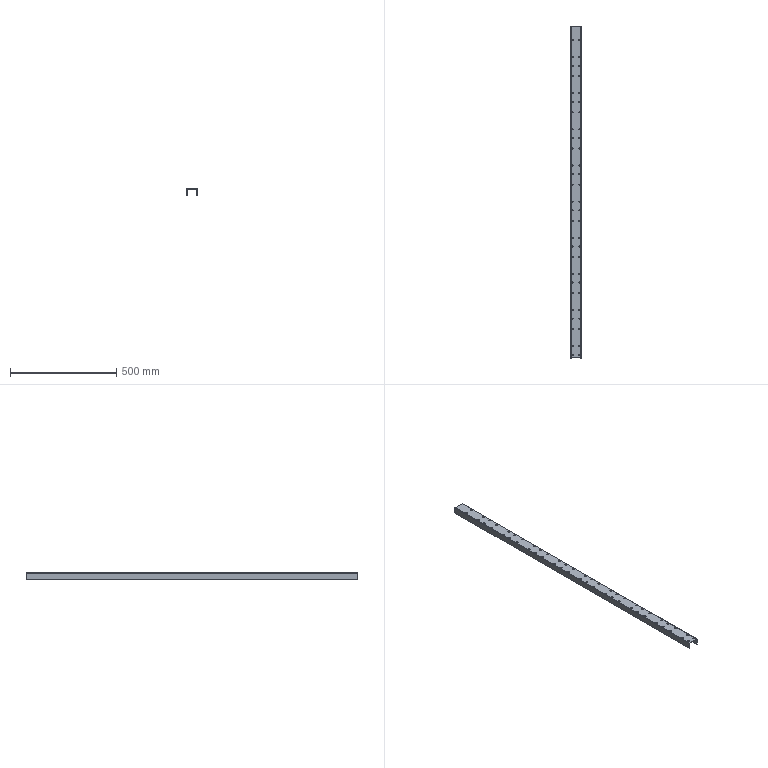Part | SolidWorks | features SplitBody 1 | 1 solid | 454 faces | box 50 x 1562 x 30 mm | volume 258598 mm3 | cylinder 328 | plane 126 | commonest cylinder face diameters 4.5 x108 5.5 x108 10.5 x108 0.2 x2 3.2 x2